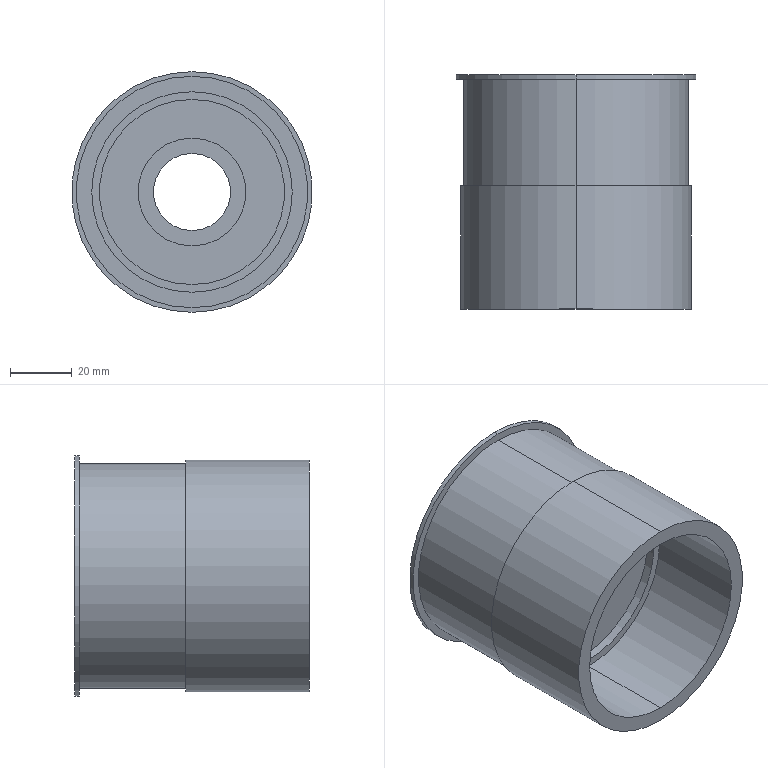Part | SolidWorks | features Revolution 1 | 1 solid | 21 faces | box 78 x 76 x 78 mm | volume 183588 mm3 | cylinder 14 | plane 7 | commonest cylinder face diameters 25 x2 35 x2 60 x2 65 x2 73 x2 75 x2
STEP:
#1=CARTESIAN_POINT('',(0.,40.,-37.5));
#2=VERTEX_POINT('',#1);
#3=CARTESIAN_POINT('',(0.,40.,37.5));
#4=VERTEX_POINT('',#3);
#5=CARTESIAN_POINT('',(0.,40.,0.));
#6=DIRECTION('',(0.,-1.,0.));
#7=DIRECTION('',(0.,0.,-1.));
#8=AXIS2_PLACEMENT_3D('',#5,#6,#7);
#9=CIRCLE('',#8,37.5);
#10=EDGE_CURVE('',#2,#4,#9,.T.);
#11=ORIENTED_EDGE('',*,*,#10,.T.);
#12=CARTESIAN_POINT('',(0.,0.,37.5));
#13=VERTEX_POINT('',#12);
#14=CARTESIAN_POINT('',(0.,0.,37.5));
#15=DIRECTION('',(0.,-1.,0.));
#16=VECTOR('',#15,1000.);
#17=LINE('',#14,#16);
#18=EDGE_CURVE('',#4,#13,#17,.T.);
#19=ORIENTED_EDGE('',*,*,#18,.T.);
#20=CARTESIAN_POINT('',(0.,0.,-37.5));
#21=VERTEX_POINT('',#20);
#22=CARTESIAN_POINT('',(0.,0.,0.));
#23=DIRECTION('',(0.,-1.,0.));
#24=DIRECTION('',(0.,0.,-1.));
#25=AXIS2_PLACEMENT_3D('',#22,#23,#24);
#26=CIRCLE('',#25,37.5);
#27=EDGE_CURVE('',#21,#13,#26,.T.);
#28=ORIENTED_EDGE('',*,*,#27,.F.);
#29=CARTESIAN_POINT('',(0.,0.,-37.5));
#30=DIRECTION('',(0.,-1.,0.));
#31=VECTOR('',#30,1000.);
#32=LINE('',#29,#31);
#33=EDGE_CURVE('',#2,#21,#32,.T.);
#34=ORIENTED_EDGE('',*,*,#33,.F.);
#35=EDGE_LOOP('',(#11,#19,#28,#34));
#36=FACE_OUTER_BOUND('',#35,.T.);
#37=CARTESIAN_POINT('',(0.,0.,0.));
#38=DIRECTION('',(0.,-1.,0.));
#39=DIRECTION('',(0.,0.,-1.));
#40=AXIS2_PLACEMENT_3D('',#37,#38,#39);
#41=CYLINDRICAL_SURFACE('',#40,37.5);
#42=ADVANCED_FACE('',(#36),#41,.T.);
#43=CARTESIAN_POINT('',(0.,74.5,-36.5));
#44=VERTEX_POINT('',#43);
#45=CARTESIAN_POINT('',(0.,74.5,36.5));
#46=VERTEX_POINT('',#45);
#47=CARTESIAN_POINT('',(0.,74.5,0.));
#48=DIRECTION('',(0.,-1.,0.));
#49=DIRECTION('',(0.,0.,-1.));
#50=AXIS2_PLACEMENT_3D('',#47,#48,#49);
#51=CIRCLE('',#50,36.5);
#52=EDGE_CURVE('',#44,#46,#51,.T.);
#53=ORIENTED_EDGE('',*,*,#52,.T.);
#54=CARTESIAN_POINT('',(0.,40.,36.5));
#55=VERTEX_POINT('',#54);
#56=CARTESIAN_POINT('',(0.,0.,36.5));
#57=DIRECTION('',(0.,-1.,0.));
#58=VECTOR('',#57,1000.);
#59=LINE('',#56,#58);
#60=EDGE_CURVE('',#46,#55,#59,.T.);
#61=ORIENTED_EDGE('',*,*,#60,.T.);
#62=CARTESIAN_POINT('',(0.,40.,-36.5));
#63=VERTEX_POINT('',#62);
#64=CARTESIAN_POINT('',(0.,40.,0.));
#65=DIRECTION('',(0.,-1.,0.));
#66=DIRECTION('',(0.,0.,-1.));
#67=AXIS2_PLACEMENT_3D('',#64,#65,#66);
#68=CIRCLE('',#67,36.5);
#69=EDGE_CURVE('',#63,#55,#68,.T.);
#70=ORIENTED_EDGE('',*,*,#69,.F.);
#71=CARTESIAN_POINT('',(0.,0.,-36.5));
#72=DIRECTION('',(0.,-1.,0.));
#73=VECTOR('',#72,1000.);
#74=LINE('',#71,#73);
#75=EDGE_CURVE('',#44,#63,#74,.T.);
#76=ORIENTED_EDGE('',*,*,#75,.F.);
#77=EDGE_LOOP('',(#53,#61,#70,#76));
#78=FACE_OUTER_BOUND('',#77,.T.);
#79=CARTESIAN_POINT('',(0.,0.,0.));
#80=DIRECTION('',(0.,-1.,0.));
#81=DIRECTION('',(0.,0.,-1.));
#82=AXIS2_PLACEMENT_3D('',#79,#80,#81);
#83=CYLINDRICAL_SURFACE('',#82,36.5);
#84=ADVANCED_FACE('',(#78),#83,.T.);
#85=CARTESIAN_POINT('',(0.,76.,-39.));
#86=VERTEX_POINT('',#85);
#87=CARTESIAN_POINT('',(0.,76.,39.));
#88=VERTEX_POINT('',#87);
#89=CARTESIAN_POINT('',(0.,76.,0.));
#90=DIRECTION('',(0.,-1.,0.));
#91=DIRECTION('',(0.,0.,-1.));
#92=AXIS2_PLACEMENT_3D('',#89,#90,#91);
#93=CIRCLE('',#92,39.);
#94=EDGE_CURVE('',#86,#88,#93,.T.);
#95=ORIENTED_EDGE('',*,*,#94,.T.);
#96=CARTESIAN_POINT('',(0.,74.5,39.));
#97=VERTEX_POINT('',#96);
#98=CARTESIAN_POINT('',(0.,0.,39.));
#99=DIRECTION('',(0.,-1.,0.));
#100=VECTOR('',#99,1000.);
#101=LINE('',#98,#100);
#102=EDGE_CURVE('',#88,#97,#101,.T.);
#103=ORIENTED_EDGE('',*,*,#102,.T.);
#104=CARTESIAN_POINT('',(0.,74.5,-39.));
#105=VERTEX_POINT('',#104);
#106=CARTESIAN_POINT('',(0.,74.5,0.));
#107=DIRECTION('',(0.,-1.,0.));
#108=DIRECTION('',(0.,0.,-1.));
#109=AXIS2_PLACEMENT_3D('',#106,#107,#108);
#110=CIRCLE('',#109,39.);
#111=EDGE_CURVE('',#105,#97,#110,.T.);
#112=ORIENTED_EDGE('',*,*,#111,.F.);
#113=CARTESIAN_POINT('',(0.,0.,-39.));
#114=DIRECTION('',(0.,-1.,0.));
#115=VECTOR('',#114,1000.);
#116=LINE('',#113,#115);
#117=EDGE_CURVE('',#86,#105,#116,.T.);
#118=ORIENTED_EDGE('',*,*,#117,.F.);
#119=EDGE_LOOP('',(#95,#103,#112,#118));
#120=FACE_OUTER_BOUND('',#119,.T.);
#121=CARTESIAN_POINT('',(0.,0.,0.));
#122=DIRECTION('',(0.,-1.,0.));
#123=DIRECTION('',(0.,0.,-1.));
#124=AXIS2_PLACEMENT_3D('',#121,#122,#123);
#125=CYLINDRICAL_SURFACE('',#124,39.);
#126=ADVANCED_FACE('',(#120),#125,.T.);
#127=CARTESIAN_POINT('',(0.,76.,12.5));
#128=VERTEX_POINT('',#127);
#129=CARTESIAN_POINT('',(0.,76.,-12.5));
#130=VERTEX_POINT('',#129);
#131=CARTESIAN_POINT('',(0.,76.,0.));
#132=DIRECTION('',(0.,-1.,0.));
#133=DIRECTION('',(0.,0.,-1.));
#134=AXIS2_PLACEMENT_3D('',#131,#132,#133);
#135=CIRCLE('',#134,12.5);
#136=EDGE_CURVE('',#128,#130,#135,.T.);
#137=ORIENTED_EDGE('',*,*,#136,.F.);
#138=CARTESIAN_POINT('',(0.,51.,12.5));
#139=VERTEX_POINT('',#138);
#140=CARTESIAN_POINT('',(0.,0.,12.5));
#141=DIRECTION('',(0.,-1.,0.));
#142=VECTOR('',#141,1000.);
#143=LINE('',#140,#142);
#144=EDGE_CURVE('',#128,#139,#143,.T.);
#145=ORIENTED_EDGE('',*,*,#144,.T.);
#146=CARTESIAN_POINT('',(0.,51.,-12.5));
#147=VERTEX_POINT('',#146);
#148=CARTESIAN_POINT('',(0.,51.,0.));
#149=DIRECTION('',(0.,-1.,0.));
#150=DIRECTION('',(0.,0.,-1.));
#151=AXIS2_PLACEMENT_3D('',#148,#149,#150);
#152=CIRCLE('',#151,12.5);
#153=EDGE_CURVE('',#139,#147,#152,.T.);
#154=ORIENTED_EDGE('',*,*,#153,.T.);
#155=CARTESIAN_POINT('',(0.,0.,-12.5));
#156=DIRECTION('',(0.,-1.,0.));
#157=VECTOR('',#156,1000.);
#158=LINE('',#155,#157);
#159=EDGE_CURVE('',#130,#147,#158,.T.);
#160=ORIENTED_EDGE('',*,*,#159,.F.);
#161=EDGE_LOOP('',(#137,#145,#154,#160));
#162=FACE_OUTER_BOUND('',#161,.T.);
#163=CARTESIAN_POINT('',(0.,0.,0.));
#164=DIRECTION('',(0.,-1.,0.));
#165=DIRECTION('',(0.,0.,-1.));
#166=AXIS2_PLACEMENT_3D('',#163,#164,#165);
#167=CYLINDRICAL_SURFACE('',#166,12.5);
#168=ADVANCED_FACE('',(#162),#167,.F.);
#169=CARTESIAN_POINT('',(0.,51.,17.5));
#170=VERTEX_POINT('',#169);
#171=CARTESIAN_POINT('',(0.,51.,-17.5));
#172=VERTEX_POINT('',#171);
#173=CARTESIAN_POINT('',(0.,51.,0.));
#174=DIRECTION('',(0.,-1.,0.));
#175=DIRECTION('',(0.,0.,-1.));
#176=AXIS2_PLACEMENT_3D('',#173,#174,#175);
#177=CIRCLE('',#176,17.5);
#178=EDGE_CURVE('',#170,#172,#177,.T.);
#179=ORIENTED_EDGE('',*,*,#178,.F.);
#180=CARTESIAN_POINT('',(0.,36.,17.5));
#181=VERTEX_POINT('',#180);
#182=CARTESIAN_POINT('',(0.,0.,17.5));
#183=DIRECTION('',(0.,-1.,0.));
#184=VECTOR('',#183,1000.);
#185=LINE('',#182,#184);
#186=EDGE_CURVE('',#170,#181,#185,.T.);
#187=ORIENTED_EDGE('',*,*,#186,.T.);
#188=CARTESIAN_POINT('',(0.,36.,-17.5));
#189=VERTEX_POINT('',#188);
#190=CARTESIAN_POINT('',(0.,36.,0.));
#191=DIRECTION('',(0.,-1.,0.));
#192=DIRECTION('',(0.,0.,-1.));
#193=AXIS2_PLACEMENT_3D('',#190,#191,#192);
#194=CIRCLE('',#193,17.5);
#195=EDGE_CURVE('',#181,#189,#194,.T.);
#196=ORIENTED_EDGE('',*,*,#195,.T.);
#197=CARTESIAN_POINT('',(0.,0.,-17.5));
#198=DIRECTION('',(0.,-1.,0.));
#199=VECTOR('',#198,1000.);
#200=LINE('',#197,#199);
#201=EDGE_CURVE('',#172,#189,#200,.T.);
#202=ORIENTED_EDGE('',*,*,#201,.F.);
#203=EDGE_LOOP('',(#179,#187,#196,#202));
#204=FACE_OUTER_BOUND('',#203,.T.);
#205=CARTESIAN_POINT('',(0.,0.,0.));
#206=DIRECTION('',(0.,-1.,0.));
#207=DIRECTION('',(0.,0.,-1.));
#208=AXIS2_PLACEMENT_3D('',#205,#206,#207);
#209=CYLINDRICAL_SURFACE('',#208,17.5);
#210=ADVANCED_FACE('',(#204),#209,.F.);
#211=CARTESIAN_POINT('',(0.,36.,30.));
#212=VERTEX_POINT('',#211);
#213=CARTESIAN_POINT('',(0.,36.,-30.));
#214=VERTEX_POINT('',#213);
#215=CARTESIAN_POINT('',(0.,36.,0.));
#216=DIRECTION('',(0.,-1.,0.));
#217=DIRECTION('',(0.,0.,-1.));
#218=AXIS2_PLACEMENT_3D('',#215,#216,#217);
#219=CIRCLE('',#218,30.);
#220=EDGE_CURVE('',#212,#214,#219,.T.);
#221=ORIENTED_EDGE('',*,*,#220,.F.);
#222=CARTESIAN_POINT('',(0.,33.,30.));
#223=VERTEX_POINT('',#222);
#224=CARTESIAN_POINT('',(0.,0.,30.));
#225=DIRECTION('',(0.,-1.,0.));
#226=VECTOR('',#225,1000.);
#227=LINE('',#224,#226);
#228=EDGE_CURVE('',#212,#223,#227,.T.);
#229=ORIENTED_EDGE('',*,*,#228,.T.);
#230=CARTESIAN_POINT('',(0.,33.,-30.));
#231=VERTEX_POINT('',#230);
#232=CARTESIAN_POINT('',(0.,33.,0.));
#233=DIRECTION('',(0.,-1.,0.));
#234=DIRECTION('',(0.,0.,-1.));
#235=AXIS2_PLACEMENT_3D('',#232,#233,#234);
#236=CIRCLE('',#235,30.);
#237=EDGE_CURVE('',#223,#231,#236,.T.);
#238=ORIENTED_EDGE('',*,*,#237,.T.);
#239=CARTESIAN_POINT('',(0.,0.,-30.));
#240=DIRECTION('',(0.,-1.,0.));
#241=VECTOR('',#240,1000.);
#242=LINE('',#239,#241);
#243=EDGE_CURVE('',#214,#231,#242,.T.);
#244=ORIENTED_EDGE('',*,*,#243,.F.);
#245=EDGE_LOOP('',(#221,#229,#238,#244));
#246=FACE_OUTER_BOUND('',#245,.T.);
#247=CARTESIAN_POINT('',(0.,0.,0.));
#248=DIRECTION('',(0.,-1.,0.));
#249=DIRECTION('',(0.,0.,-1.));
#250=AXIS2_PLACEMENT_3D('',#247,#248,#249);
#251=CYLINDRICAL_SURFACE('',#250,30.);
#252=ADVANCED_FACE('',(#246),#251,.F.);
#253=CARTESIAN_POINT('',(0.,33.,32.5));
#254=VERTEX_POINT('',#253);
#255=CARTESIAN_POINT('',(0.,33.,-32.5));
#256=VERTEX_POINT('',#255);
#257=CARTESIAN_POINT('',(0.,33.,0.));
#258=DIRECTION('',(0.,-1.,0.));
#259=DIRECTION('',(0.,0.,-1.));
#260=AXIS2_PLACEMENT_3D('',#257,#258,#259);
#261=CIRCLE('',#260,32.5);
#262=EDGE_CURVE('',#254,#256,#261,.T.);
#263=ORIENTED_EDGE('',*,*,#262,.F.);
#264=CARTESIAN_POINT('',(0.,0.,32.5));
#265=VERTEX_POINT('',#264);
#266=CARTESIAN_POINT('',(0.,0.,32.5));
#267=DIRECTION('',(0.,-1.,0.));
#268=VECTOR('',#267,1000.);
#269=LINE('',#266,#268);
#270=EDGE_CURVE('',#254,#265,#269,.T.);
#271=ORIENTED_EDGE('',*,*,#270,.T.);
#272=CARTESIAN_POINT('',(0.,0.,-32.5));
#273=VERTEX_POINT('',#272);
#274=CARTESIAN_POINT('',(0.,0.,0.));
#275=DIRECTION('',(0.,-1.,0.));
#276=DIRECTION('',(0.,0.,-1.));
#277=AXIS2_PLACEMENT_3D('',#274,#275,#276);
#278=CIRCLE('',#277,32.5);
#279=EDGE_CURVE('',#265,#273,#278,.T.);
#280=ORIENTED_EDGE('',*,*,#279,.T.);
#281=CARTESIAN_POINT('',(0.,0.,-32.5));
#282=DIRECTION('',(0.,-1.,0.));
#283=VECTOR('',#282,1000.);
#284=LINE('',#281,#283);
#285=EDGE_CURVE('',#256,#273,#284,.T.);
#286=ORIENTED_EDGE('',*,*,#285,.F.);
#287=EDGE_LOOP('',(#263,#271,#280,#286));
#288=FACE_OUTER_BOUND('',#287,.T.);
#289=CARTESIAN_POINT('',(0.,0.,0.));
#290=DIRECTION('',(0.,-1.,0.));
#291=DIRECTION('',(0.,0.,-1.));
#292=AXIS2_PLACEMENT_3D('',#289,#290,#291);
#293=CYLINDRICAL_SURFACE('',#292,32.5);
#294=ADVANCED_FACE('',(#288),#293,.F.);
#295=CARTESIAN_POINT('',(0.,0.,0.));
#296=DIRECTION('',(0.,-1.,0.));
#297=DIRECTION('',(0.,0.,-1.));
#298=AXIS2_PLACEMENT_3D('',#295,#296,#297);
#299=CIRCLE('',#298,32.5);
#300=EDGE_CURVE('',#273,#265,#299,.T.);
#301=ORIENTED_EDGE('',*,*,#300,.F.);
#302=ORIENTED_EDGE('',*,*,#279,.F.);
#303=EDGE_LOOP('',(#301,#302));
#304=FACE_BOUND('',#303,.T.);
#305=ORIENTED_EDGE('',*,*,#27,.T.);
#306=CARTESIAN_POINT('',(0.,0.,0.));
#307=DIRECTION('',(0.,-1.,0.));
#308=DIRECTION('',(0.,0.,-1.));
#309=AXIS2_PLACEMENT_3D('',#306,#307,#308);
#310=CIRCLE('',#309,37.5);
#311=EDGE_CURVE('',#13,#21,#310,.T.);
#312=ORIENTED_EDGE('',*,*,#311,.T.);
#313=EDGE_LOOP('',(#305,#312));
#314=FACE_OUTER_BOUND('',#313,.T.);
#315=CARTESIAN_POINT('',(-37.5,0.,0.));
#316=DIRECTION('',(0.,1.,0.));
#317=DIRECTION('',(0.,0.,1.));
#318=AXIS2_PLACEMENT_3D('',#315,#316,#317);
#319=PLANE('',#318);
#320=ADVANCED_FACE('',(#304,#314),#319,.F.);
#321=ORIENTED_EDGE('',*,*,#270,.F.);
#322=CARTESIAN_POINT('',(0.,33.,0.));
#323=DIRECTION('',(0.,-1.,0.));
#324=DIRECTION('',(0.,0.,-1.));
#325=AXIS2_PLACEMENT_3D('',#322,#323,#324);
#326=CIRCLE('',#325,32.5);
#327=EDGE_CURVE('',#256,#254,#326,.T.);
#328=ORIENTED_EDGE('',*,*,#327,.F.);
#329=ORIENTED_EDGE('',*,*,#285,.T.);
#330=ORIENTED_EDGE('',*,*,#300,.T.);
#331=EDGE_LOOP('',(#321,#328,#329,#330));
#332=FACE_OUTER_BOUND('',#331,.T.);
#333=CARTESIAN_POINT('',(0.,0.,0.));
#334=DIRECTION('',(0.,-1.,0.));
#335=DIRECTION('',(0.,0.,-1.));
#336=AXIS2_PLACEMENT_3D('',#333,#334,#335);
#337=CYLINDRICAL_SURFACE('',#336,32.5);
#338=ADVANCED_FACE('',(#332),#337,.F.);
#339=CARTESIAN_POINT('',(0.,33.,0.));
#340=DIRECTION('',(0.,-1.,0.));
#341=DIRECTION('',(0.,0.,-1.));
#342=AXIS2_PLACEMENT_3D('',#339,#340,#341);
#343=CIRCLE('',#342,30.);
#344=EDGE_CURVE('',#231,#223,#343,.T.);
#345=ORIENTED_EDGE('',*,*,#344,.F.);
#346=ORIENTED_EDGE('',*,*,#237,.F.);
#347=EDGE_LOOP('',(#345,#346));
#348=FACE_BOUND('',#347,.T.);
#349=ORIENTED_EDGE('',*,*,#327,.T.);
#350=ORIENTED_EDGE('',*,*,#262,.T.);
#351=EDGE_LOOP('',(#349,#350));
#352=FACE_OUTER_BOUND('',#351,.T.);
#353=CARTESIAN_POINT('',(-32.5,33.,0.));
#354=DIRECTION('',(0.,1.,0.));
#355=DIRECTION('',(0.,0.,1.));
#356=AXIS2_PLACEMENT_3D('',#353,#354,#355);
#357=PLANE('',#356);
#358=ADVANCED_FACE('',(#348,#352),#357,.F.);
#359=ORIENTED_EDGE('',*,*,#228,.F.);
#360=CARTESIAN_POINT('',(0.,36.,0.));
#361=DIRECTION('',(0.,-1.,0.));
#362=DIRECTION('',(0.,0.,-1.));
#363=AXIS2_PLACEMENT_3D('',#360,#361,#362);
#364=CIRCLE('',#363,30.);
#365=EDGE_CURVE('',#214,#212,#364,.T.);
#366=ORIENTED_EDGE('',*,*,#365,.F.);
#367=ORIENTED_EDGE('',*,*,#243,.T.);
#368=ORIENTED_EDGE('',*,*,#344,.T.);
#369=EDGE_LOOP('',(#359,#366,#367,#368));
#370=FACE_OUTER_BOUND('',#369,.T.);
#371=CARTESIAN_POINT('',(0.,0.,0.));
#372=DIRECTION('',(0.,-1.,0.));
#373=DIRECTION('',(0.,0.,-1.));
#374=AXIS2_PLACEMENT_3D('',#371,#372,#373);
#375=CYLINDRICAL_SURFACE('',#374,30.);
#376=ADVANCED_FACE('',(#370),#375,.F.);
#377=CARTESIAN_POINT('',(0.,36.,0.));
#378=DIRECTION('',(0.,-1.,0.));
#379=DIRECTION('',(0.,0.,-1.));
#380=AXIS2_PLACEMENT_3D('',#377,#378,#379);
#381=CIRCLE('',#380,17.5);
#382=EDGE_CURVE('',#189,#181,#381,.T.);
#383=ORIENTED_EDGE('',*,*,#382,.F.);
#384=ORIENTED_EDGE('',*,*,#195,.F.);
#385=EDGE_LOOP('',(#383,#384));
#386=FACE_BOUND('',#385,.T.);
#387=ORIENTED_EDGE('',*,*,#365,.T.);
#388=ORIENTED_EDGE('',*,*,#220,.T.);
#389=EDGE_LOOP('',(#387,#388));
#390=FACE_OUTER_BOUND('',#389,.T.);
#391=CARTESIAN_POINT('',(-30.,36.,0.));
#392=DIRECTION('',(0.,1.,0.));
#393=DIRECTION('',(0.,0.,1.));
#394=AXIS2_PLACEMENT_3D('',#391,#392,#393);
#395=PLANE('',#394);
#396=ADVANCED_FACE('',(#386,#390),#395,.F.);
#397=ORIENTED_EDGE('',*,*,#186,.F.);
#398=CARTESIAN_POINT('',(0.,51.,0.));
#399=DIRECTION('',(0.,-1.,0.));
#400=DIRECTION('',(0.,0.,-1.));
#401=AXIS2_PLACEMENT_3D('',#398,#399,#400);
#402=CIRCLE('',#401,17.5);
#403=EDGE_CURVE('',#172,#170,#402,.T.);
#404=ORIENTED_EDGE('',*,*,#403,.F.);
#405=ORIENTED_EDGE('',*,*,#201,.T.);
#406=ORIENTED_EDGE('',*,*,#382,.T.);
#407=EDGE_LOOP('',(#397,#404,#405,#406));
#408=FACE_OUTER_BOUND('',#407,.T.);
#409=CARTESIAN_POINT('',(0.,0.,0.));
#410=DIRECTION('',(0.,-1.,0.));
#411=DIRECTION('',(0.,0.,-1.));
#412=AXIS2_PLACEMENT_3D('',#409,#410,#411);
#413=CYLINDRICAL_SURFACE('',#412,17.5);
#414=ADVANCED_FACE('',(#408),#413,.F.);
#415=CARTESIAN_POINT('',(0.,51.,0.));
#416=DIRECTION('',(0.,-1.,0.));
#417=DIRECTION('',(0.,0.,-1.));
#418=AXIS2_PLACEMENT_3D('',#415,#416,#417);
#419=CIRCLE('',#418,12.5);
#420=EDGE_CURVE('',#147,#139,#419,.T.);
#421=ORIENTED_EDGE('',*,*,#420,.F.);
#422=ORIENTED_EDGE('',*,*,#153,.F.);
#423=EDGE_LOOP('',(#421,#422));
#424=FACE_BOUND('',#423,.T.);
#425=ORIENTED_EDGE('',*,*,#403,.T.);
#426=ORIENTED_EDGE('',*,*,#178,.T.);
#427=EDGE_LOOP('',(#425,#426));
#428=FACE_OUTER_BOUND('',#427,.T.);
#429=CARTESIAN_POINT('',(-17.5,51.,0.));
#430=DIRECTION('',(0.,1.,0.));
#431=DIRECTION('',(0.,0.,1.));
#432=AXIS2_PLACEMENT_3D('',#429,#430,#431);
#433=PLANE('',#432);
#434=ADVANCED_FACE('',(#424,#428),#433,.F.);
#435=ORIENTED_EDGE('',*,*,#144,.F.);
#436=CARTESIAN_POINT('',(0.,76.,0.));
#437=DIRECTION('',(0.,-1.,0.));
#438=DIRECTION('',(0.,0.,-1.));
#439=AXIS2_PLACEMENT_3D('',#436,#437,#438);
#440=CIRCLE('',#439,12.5);
#441=EDGE_CURVE('',#130,#128,#440,.T.);
#442=ORIENTED_EDGE('',*,*,#441,.F.);
#443=ORIENTED_EDGE('',*,*,#159,.T.);
#444=ORIENTED_EDGE('',*,*,#420,.T.);
#445=EDGE_LOOP('',(#435,#442,#443,#444));
#446=FACE_OUTER_BOUND('',#445,.T.);
#447=CARTESIAN_POINT('',(0.,0.,0.));
#448=DIRECTION('',(0.,-1.,0.));
#449=DIRECTION('',(0.,0.,-1.));
#450=AXIS2_PLACEMENT_3D('',#447,#448,#449);
#451=CYLINDRICAL_SURFACE('',#450,12.5);
#452=ADVANCED_FACE('',(#446),#451,.F.);
#453=ORIENTED_EDGE('',*,*,#94,.F.);
#454=CARTESIAN_POINT('',(0.,76.,0.));
#455=DIRECTION('',(0.,-1.,0.));
#456=DIRECTION('',(0.,0.,-1.));
#457=AXIS2_PLACEMENT_3D('',#454,#455,#456);
#458=CIRCLE('',#457,39.);
#459=EDGE_CURVE('',#88,#86,#458,.T.);
#460=ORIENTED_EDGE('',*,*,#459,.F.);
#461=EDGE_LOOP('',(#453,#460));
#462=FACE_OUTER_BOUND('',#461,.T.);
#463=ORIENTED_EDGE('',*,*,#441,.T.);
#464=ORIENTED_EDGE('',*,*,#136,.T.);
#465=EDGE_LOOP('',(#463,#464));
#466=FACE_BOUND('',#465,.T.);
#467=CARTESIAN_POINT('',(-39.,76.,0.));
#468=DIRECTION('',(0.,-1.,0.));
#469=DIRECTION('',(0.,0.,-1.));
#470=AXIS2_PLACEMENT_3D('',#467,#468,#469);
#471=PLANE('',#470);
#472=ADVANCED_FACE('',(#462,#466),#471,.F.);
#473=ORIENTED_EDGE('',*,*,#102,.F.);
#474=ORIENTED_EDGE('',*,*,#459,.T.);
#475=ORIENTED_EDGE('',*,*,#117,.T.);
#476=CARTESIAN_POINT('',(0.,74.5,0.));
#477=DIRECTION('',(0.,-1.,0.));
#478=DIRECTION('',(0.,0.,-1.));
#479=AXIS2_PLACEMENT_3D('',#476,#477,#478);
#480=CIRCLE('',#479,39.);
#481=EDGE_CURVE('',#97,#105,#480,.T.);
#482=ORIENTED_EDGE('',*,*,#481,.F.);
#483=EDGE_LOOP('',(#473,#474,#475,#482));
#484=FACE_OUTER_BOUND('',#483,.T.);
#485=CARTESIAN_POINT('',(0.,0.,0.));
#486=DIRECTION('',(0.,-1.,0.));
#487=DIRECTION('',(0.,0.,-1.));
#488=AXIS2_PLACEMENT_3D('',#485,#486,#487);
#489=CYLINDRICAL_SURFACE('',#488,39.);
#490=ADVANCED_FACE('',(#484),#489,.T.);
#491=ORIENTED_EDGE('',*,*,#52,.F.);
#492=CARTESIAN_POINT('',(0.,74.5,0.));
#493=DIRECTION('',(0.,-1.,0.));
#494=DIRECTION('',(0.,0.,-1.));
#495=AXIS2_PLACEMENT_3D('',#492,#493,#494);
#496=CIRCLE('',#495,36.5);
#497=EDGE_CURVE('',#46,#44,#496,.T.);
#498=ORIENTED_EDGE('',*,*,#497,.F.);
#499=EDGE_LOOP('',(#491,#498));
#500=FACE_BOUND('',#499,.T.);
#501=ORIENTED_EDGE('',*,*,#111,.T.);
#502=ORIENTED_EDGE('',*,*,#481,.T.);
#503=EDGE_LOOP('',(#501,#502));
#504=FACE_OUTER_BOUND('',#503,.T.);
#505=CARTESIAN_POINT('',(-36.5,74.5,0.));
#506=DIRECTION('',(0.,1.,0.));
#507=DIRECTION('',(0.,0.,1.));
#508=AXIS2_PLACEMENT_3D('',#505,#506,#507);
#509=PLANE('',#508);
#510=ADVANCED_FACE('',(#500,#504),#509,.F.);
#511=ORIENTED_EDGE('',*,*,#60,.F.);
#512=ORIENTED_EDGE('',*,*,#497,.T.);
#513=ORIENTED_EDGE('',*,*,#75,.T.);
#514=CARTESIAN_POINT('',(0.,40.,0.));
#515=DIRECTION('',(0.,-1.,0.));
#516=DIRECTION('',(0.,0.,-1.));
#517=AXIS2_PLACEMENT_3D('',#514,#515,#516);
#518=CIRCLE('',#517,36.5);
#519=EDGE_CURVE('',#55,#63,#518,.T.);
#520=ORIENTED_EDGE('',*,*,#519,.F.);
#521=EDGE_LOOP('',(#511,#512,#513,#520));
#522=FACE_OUTER_BOUND('',#521,.T.);
#523=CARTESIAN_POINT('',(0.,0.,0.));
#524=DIRECTION('',(0.,-1.,0.));
#525=DIRECTION('',(0.,0.,-1.));
#526=AXIS2_PLACEMENT_3D('',#523,#524,#525);
#527=CYLINDRICAL_SURFACE('',#526,36.5);
#528=ADVANCED_FACE('',(#522),#527,.T.);
#529=ORIENTED_EDGE('',*,*,#10,.F.);
#530=CARTESIAN_POINT('',(0.,40.,0.));
#531=DIRECTION('',(0.,-1.,0.));
#532=DIRECTION('',(0.,0.,-1.));
#533=AXIS2_PLACEMENT_3D('',#530,#531,#532);
#534=CIRCLE('',#533,37.5);
#535=EDGE_CURVE('',#4,#2,#534,.T.);
#536=ORIENTED_EDGE('',*,*,#535,.F.);
#537=EDGE_LOOP('',(#529,#536));
#538=FACE_OUTER_BOUND('',#537,.T.);
#539=ORIENTED_EDGE('',*,*,#69,.T.);
#540=ORIENTED_EDGE('',*,*,#519,.T.);
#541=EDGE_LOOP('',(#539,#540));
#542=FACE_BOUND('',#541,.T.);
#543=CARTESIAN_POINT('',(-37.5,40.,0.));
#544=DIRECTION('',(0.,-1.,0.));
#545=DIRECTION('',(0.,0.,-1.));
#546=AXIS2_PLACEMENT_3D('',#543,#544,#545);
#547=PLANE('',#546);
#548=ADVANCED_FACE('',(#538,#542),#547,.F.);
#549=ORIENTED_EDGE('',*,*,#18,.F.);
#550=ORIENTED_EDGE('',*,*,#535,.T.);
#551=ORIENTED_EDGE('',*,*,#33,.T.);
#552=ORIENTED_EDGE('',*,*,#311,.F.);
#553=EDGE_LOOP('',(#549,#550,#551,#552));
#554=FACE_OUTER_BOUND('',#553,.T.);
#555=CARTESIAN_POINT('',(0.,0.,0.));
#556=DIRECTION('',(0.,-1.,0.));
#557=DIRECTION('',(0.,0.,-1.));
#558=AXIS2_PLACEMENT_3D('',#555,#556,#557);
#559=CYLINDRICAL_SURFACE('',#558,37.5);
#560=ADVANCED_FACE('',(#554),#559,.T.);
#561=CLOSED_SHELL('',(#42,#84,#126,#168,#210,#252,#294,#320,#338,#358,#376,#396,#414,#434,#452,#472,#490,#510,#528,#548,#560));
#562=MANIFOLD_SOLID_BREP('',#561);
#563=CARTESIAN_POINT('',(0.,0.,0.));
#564=DIRECTION('',(0.,0.,1.));
#565=DIRECTION('',(1.,0.,0.));
#566=AXIS2_PLACEMENT_3D('',#563,#564,#565);
#567=(LENGTH_UNIT()NAMED_UNIT(*)SI_UNIT(.MILLI.,.METRE.));
#568=UNCERTAINTY_MEASURE_WITH_UNIT(LENGTH_MEASURE(0.00001),#567,'','');
#569=(NAMED_UNIT(*)PLANE_ANGLE_UNIT()SI_UNIT($,.RADIAN.));
#570=(NAMED_UNIT(*)SI_UNIT($,.STERADIAN.)SOLID_ANGLE_UNIT());
#571=(GEOMETRIC_REPRESENTATION_CONTEXT(3)GLOBAL_UNCERTAINTY_ASSIGNED_CONTEXT((#568))GLOBAL_UNIT_ASSIGNED_CONTEXT((#567,#569,#570))REPRESENTATION_CONTEXT('',''));
#572=ADVANCED_BREP_SHAPE_REPRESENTATION('',(#562,#566),#571);